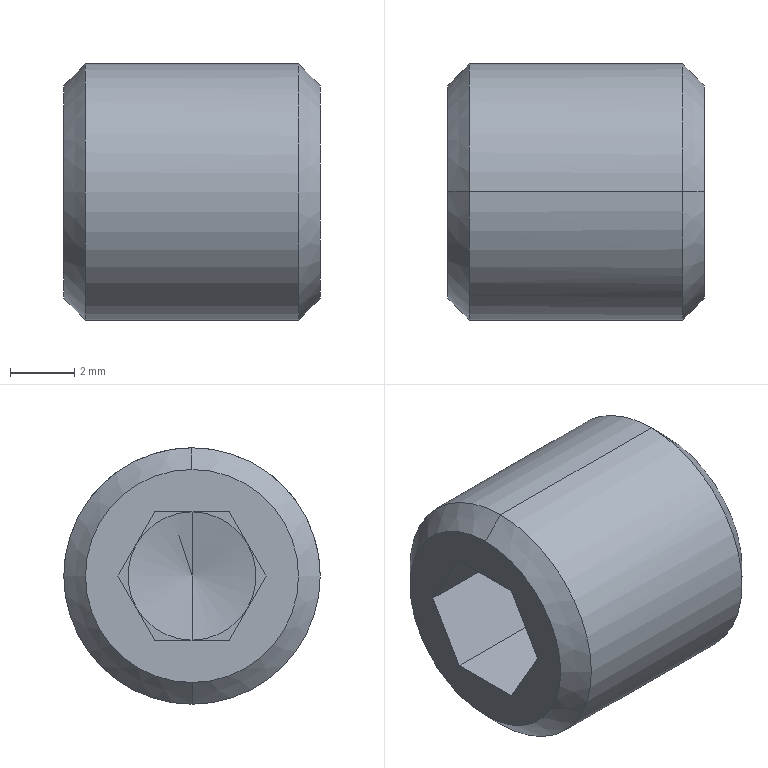Part | STEP file | _MSW8 | 1 solid | 22 faces | box 8 x 8 x 8 mm | volume 320.313 mm3 | plane 14 | cone 6 | cylinder 2 | commonest cylinder face diameters 8 x2
STEP:
#1=CARTESIAN_POINT('',(1.,0.,2.));
#2=VERTEX_POINT('',#1);
#3=CARTESIAN_POINT('',(1.,1.732,1.));
#4=VERTEX_POINT('',#3);
#5=CARTESIAN_POINT('',(1.,0.,0.));
#6=DIRECTION('',(-1.,0.,0.));
#7=AXIS2_PLACEMENT_3D('',#5,#6,$);
#8=CIRCLE('',#7,2.);
#9=EDGE_CURVE('',#2,#4,#8,.T.);
#10=ORIENTED_EDGE('',*,*,#9,.T.);
#11=CARTESIAN_POINT('',(1.,1.732,-1.));
#12=VERTEX_POINT('',#11);
#13=CARTESIAN_POINT('',(1.,0.,0.));
#14=DIRECTION('',(-1.,0.,0.));
#15=AXIS2_PLACEMENT_3D('',#13,#14,$);
#16=CIRCLE('',#15,2.);
#17=EDGE_CURVE('',#4,#12,#16,.T.);
#18=ORIENTED_EDGE('',*,*,#17,.T.);
#19=CARTESIAN_POINT('',(1.,0.,-2.));
#20=VERTEX_POINT('',#19);
#21=CARTESIAN_POINT('',(1.,0.,0.));
#22=DIRECTION('',(-1.,0.,0.));
#23=AXIS2_PLACEMENT_3D('',#21,#22,$);
#24=CIRCLE('',#23,2.);
#25=EDGE_CURVE('',#12,#20,#24,.T.);
#26=ORIENTED_EDGE('',*,*,#25,.T.);
#27=CARTESIAN_POINT('',(1.4,0.,0.));
#28=VERTEX_POINT('',#27);
#29=CARTESIAN_POINT('',(-98056.868,0.,-490291.338));
#30=DIRECTION('',(-0.1961,0.,-0.9806));
#31=VECTOR('',#30,1.);
#32=LINE('',#29,#31);
#33=EDGE_CURVE('',#28,#20,#32,.T.);
#34=ORIENTED_EDGE('',*,*,#33,.F.);
#35=CARTESIAN_POINT('',(-98056.868,0.,490291.338));
#36=DIRECTION('',(-0.1961,0.,0.9806));
#37=VECTOR('',#36,1.);
#38=LINE('',#35,#37);
#39=EDGE_CURVE('',#2,#28,#38,.F.);
#40=ORIENTED_EDGE('',*,*,#39,.F.);
#41=EDGE_LOOP('',(#10,#18,#26,#34,#40));
#42=FACE_OUTER_BOUND('',#41,.T.);
#43=CARTESIAN_POINT('',(1.,0.,0.));
#44=DIRECTION('',(-1.,0.,0.));
#45=DIRECTION('',(0.,0.,1.));
#46=AXIS2_PLACEMENT_3D('',#43,#44,#45);
#47=CONICAL_SURFACE('',#46,2.,1.373);
#48=ADVANCED_FACE('',(#42),#47,.F.);
#49=ORIENTED_EDGE('',*,*,#9,.F.);
#50=CARTESIAN_POINT('',(1.,1.155,2.));
#51=VERTEX_POINT('',#50);
#52=CARTESIAN_POINT('',(1.,0.5774,2.));
#53=DIRECTION('',(0.,-1.,0.));
#54=VECTOR('',#53,1.);
#55=LINE('',#52,#54);
#56=EDGE_CURVE('',#51,#2,#55,.T.);
#57=ORIENTED_EDGE('',*,*,#56,.F.);
#58=CARTESIAN_POINT('',(1.,1.443,1.5));
#59=DIRECTION('',(0.,-0.5,0.866));
#60=VECTOR('',#59,1.);
#61=LINE('',#58,#60);
#62=EDGE_CURVE('',#4,#51,#61,.T.);
#63=ORIENTED_EDGE('',*,*,#62,.F.);
#64=EDGE_LOOP('',(#49,#57,#63));
#65=FACE_OUTER_BOUND('',#64,.T.);
#66=CARTESIAN_POINT('',(1.,0.,0.));
#67=DIRECTION('',(1.,0.,0.));
#68=DIRECTION('',(0.,0.,-1.));
#69=AXIS2_PLACEMENT_3D('',#66,#67,#68);
#70=PLANE('',#69);
#71=ADVANCED_FACE('',(#65),#70,.F.);
#72=ORIENTED_EDGE('',*,*,#17,.F.);
#73=CARTESIAN_POINT('',(1.,2.309,0.));
#74=VERTEX_POINT('',#73);
#75=CARTESIAN_POINT('',(1.,2.021,0.5));
#76=DIRECTION('',(0.,-0.5,0.866));
#77=VECTOR('',#76,1.);
#78=LINE('',#75,#77);
#79=EDGE_CURVE('',#74,#4,#78,.T.);
#80=ORIENTED_EDGE('',*,*,#79,.F.);
#81=CARTESIAN_POINT('',(1.,2.021,-0.5));
#82=DIRECTION('',(0.,0.5,0.866));
#83=VECTOR('',#82,1.);
#84=LINE('',#81,#83);
#85=EDGE_CURVE('',#12,#74,#84,.T.);
#86=ORIENTED_EDGE('',*,*,#85,.F.);
#87=EDGE_LOOP('',(#72,#80,#86));
#88=FACE_OUTER_BOUND('',#87,.T.);
#89=CARTESIAN_POINT('',(1.,0.,0.));
#90=DIRECTION('',(1.,0.,0.));
#91=DIRECTION('',(0.,0.,-1.));
#92=AXIS2_PLACEMENT_3D('',#89,#90,#91);
#93=PLANE('',#92);
#94=ADVANCED_FACE('',(#88),#93,.F.);
#95=ORIENTED_EDGE('',*,*,#25,.F.);
#96=CARTESIAN_POINT('',(1.,1.155,-2.));
#97=VERTEX_POINT('',#96);
#98=CARTESIAN_POINT('',(1.,1.443,-1.5));
#99=DIRECTION('',(0.,0.5,0.866));
#100=VECTOR('',#99,1.);
#101=LINE('',#98,#100);
#102=EDGE_CURVE('',#97,#12,#101,.T.);
#103=ORIENTED_EDGE('',*,*,#102,.F.);
#104=CARTESIAN_POINT('',(1.,0.5774,-2.));
#105=DIRECTION('',(0.,1.,0.));
#106=VECTOR('',#105,1.);
#107=LINE('',#104,#106);
#108=EDGE_CURVE('',#20,#97,#107,.T.);
#109=ORIENTED_EDGE('',*,*,#108,.F.);
#110=EDGE_LOOP('',(#95,#103,#109));
#111=FACE_OUTER_BOUND('',#110,.T.);
#112=CARTESIAN_POINT('',(1.,0.,0.));
#113=DIRECTION('',(1.,0.,0.));
#114=DIRECTION('',(0.,0.,-1.));
#115=AXIS2_PLACEMENT_3D('',#112,#113,#114);
#116=PLANE('',#115);
#117=ADVANCED_FACE('',(#111),#116,.F.);
#118=CARTESIAN_POINT('',(1.,-1.732,-1.));
#119=VERTEX_POINT('',#118);
#120=CARTESIAN_POINT('',(1.,0.,0.));
#121=DIRECTION('',(-1.,0.,0.));
#122=AXIS2_PLACEMENT_3D('',#120,#121,$);
#123=CIRCLE('',#122,2.);
#124=EDGE_CURVE('',#20,#119,#123,.T.);
#125=ORIENTED_EDGE('',*,*,#124,.T.);
#126=CARTESIAN_POINT('',(1.,-1.732,1.));
#127=VERTEX_POINT('',#126);
#128=CARTESIAN_POINT('',(1.,0.,0.));
#129=DIRECTION('',(-1.,0.,0.));
#130=AXIS2_PLACEMENT_3D('',#128,#129,$);
#131=CIRCLE('',#130,2.);
#132=EDGE_CURVE('',#119,#127,#131,.T.);
#133=ORIENTED_EDGE('',*,*,#132,.T.);
#134=CARTESIAN_POINT('',(1.,0.,0.));
#135=DIRECTION('',(-1.,0.,0.));
#136=AXIS2_PLACEMENT_3D('',#134,#135,$);
#137=CIRCLE('',#136,2.);
#138=EDGE_CURVE('',#127,#2,#137,.T.);
#139=ORIENTED_EDGE('',*,*,#138,.T.);
#140=ORIENTED_EDGE('',*,*,#39,.T.);
#141=ORIENTED_EDGE('',*,*,#33,.T.);
#142=EDGE_LOOP('',(#125,#133,#139,#140,#141));
#143=FACE_OUTER_BOUND('',#142,.T.);
#144=CARTESIAN_POINT('',(1.,0.,0.));
#145=DIRECTION('',(-1.,0.,0.));
#146=DIRECTION('',(0.,0.,-1.));
#147=AXIS2_PLACEMENT_3D('',#144,#145,#146);
#148=CONICAL_SURFACE('',#147,2.,1.373);
#149=ADVANCED_FACE('',(#143),#148,.F.);
#150=CARTESIAN_POINT('',(-4.,1.155,2.));
#151=VERTEX_POINT('',#150);
#152=CARTESIAN_POINT('',(-4.,-1.155,2.));
#153=VERTEX_POINT('',#152);
#154=CARTESIAN_POINT('',(-4.,0.,2.));
#155=DIRECTION('',(0.,-1.,0.));
#156=VECTOR('',#155,1.);
#157=LINE('',#154,#156);
#158=EDGE_CURVE('',#151,#153,#157,.T.);
#159=ORIENTED_EDGE('',*,*,#158,.F.);
#160=CARTESIAN_POINT('',(-1.5,1.155,2.));
#161=DIRECTION('',(-1.,0.,0.));
#162=VECTOR('',#161,1.);
#163=LINE('',#160,#162);
#164=EDGE_CURVE('',#51,#151,#163,.T.);
#165=ORIENTED_EDGE('',*,*,#164,.F.);
#166=ORIENTED_EDGE('',*,*,#56,.T.);
#167=CARTESIAN_POINT('',(1.,-1.155,2.));
#168=VERTEX_POINT('',#167);
#169=CARTESIAN_POINT('',(1.,-0.5774,2.));
#170=DIRECTION('',(0.,-1.,0.));
#171=VECTOR('',#170,1.);
#172=LINE('',#169,#171);
#173=EDGE_CURVE('',#2,#168,#172,.T.);
#174=ORIENTED_EDGE('',*,*,#173,.T.);
#175=CARTESIAN_POINT('',(-1.5,-1.155,2.));
#176=DIRECTION('',(-1.,0.,0.));
#177=VECTOR('',#176,1.);
#178=LINE('',#175,#177);
#179=EDGE_CURVE('',#168,#153,#178,.T.);
#180=ORIENTED_EDGE('',*,*,#179,.T.);
#181=EDGE_LOOP('',(#159,#165,#166,#174,#180));
#182=FACE_OUTER_BOUND('',#181,.T.);
#183=CARTESIAN_POINT('',(1.,1.155,2.));
#184=DIRECTION('',(0.,0.,-1.));
#185=DIRECTION('',(-1.,0.,0.));
#186=AXIS2_PLACEMENT_3D('',#183,#184,#185);
#187=PLANE('',#186);
#188=ADVANCED_FACE('',(#182),#187,.T.);
#189=CARTESIAN_POINT('',(-4.,2.309,0.));
#190=VERTEX_POINT('',#189);
#191=CARTESIAN_POINT('',(-4.,1.732,1.));
#192=DIRECTION('',(0.,-0.5,0.866));
#193=VECTOR('',#192,1.);
#194=LINE('',#191,#193);
#195=EDGE_CURVE('',#190,#151,#194,.T.);
#196=ORIENTED_EDGE('',*,*,#195,.F.);
#197=CARTESIAN_POINT('',(-1.5,2.309,0.));
#198=DIRECTION('',(-1.,0.,0.));
#199=VECTOR('',#198,1.);
#200=LINE('',#197,#199);
#201=EDGE_CURVE('',#74,#190,#200,.T.);
#202=ORIENTED_EDGE('',*,*,#201,.F.);
#203=ORIENTED_EDGE('',*,*,#79,.T.);
#204=ORIENTED_EDGE('',*,*,#62,.T.);
#205=ORIENTED_EDGE('',*,*,#164,.T.);
#206=EDGE_LOOP('',(#196,#202,#203,#204,#205));
#207=FACE_OUTER_BOUND('',#206,.T.);
#208=CARTESIAN_POINT('',(1.,2.309,0.));
#209=DIRECTION('',(0.,-0.866,-0.5));
#210=DIRECTION('',(0.,0.5,-0.866));
#211=AXIS2_PLACEMENT_3D('',#208,#209,#210);
#212=PLANE('',#211);
#213=ADVANCED_FACE('',(#207),#212,.T.);
#214=CARTESIAN_POINT('',(-4.,1.155,-2.));
#215=VERTEX_POINT('',#214);
#216=CARTESIAN_POINT('',(-4.,1.732,-1.));
#217=DIRECTION('',(0.,0.5,0.866));
#218=VECTOR('',#217,1.);
#219=LINE('',#216,#218);
#220=EDGE_CURVE('',#215,#190,#219,.T.);
#221=ORIENTED_EDGE('',*,*,#220,.F.);
#222=CARTESIAN_POINT('',(-1.5,1.155,-2.));
#223=DIRECTION('',(-1.,0.,0.));
#224=VECTOR('',#223,1.);
#225=LINE('',#222,#224);
#226=EDGE_CURVE('',#97,#215,#225,.T.);
#227=ORIENTED_EDGE('',*,*,#226,.F.);
#228=ORIENTED_EDGE('',*,*,#102,.T.);
#229=ORIENTED_EDGE('',*,*,#85,.T.);
#230=ORIENTED_EDGE('',*,*,#201,.T.);
#231=EDGE_LOOP('',(#221,#227,#228,#229,#230));
#232=FACE_OUTER_BOUND('',#231,.T.);
#233=CARTESIAN_POINT('',(1.,1.155,-2.));
#234=DIRECTION('',(0.,-0.866,0.5));
#235=DIRECTION('',(0.,-0.5,-0.866));
#236=AXIS2_PLACEMENT_3D('',#233,#234,#235);
#237=PLANE('',#236);
#238=ADVANCED_FACE('',(#232),#237,.T.);
#239=CARTESIAN_POINT('',(-4.,-1.155,-2.));
#240=VERTEX_POINT('',#239);
#241=CARTESIAN_POINT('',(-4.,0.,-2.));
#242=DIRECTION('',(0.,1.,0.));
#243=VECTOR('',#242,1.);
#244=LINE('',#241,#243);
#245=EDGE_CURVE('',#240,#215,#244,.T.);
#246=ORIENTED_EDGE('',*,*,#245,.F.);
#247=CARTESIAN_POINT('',(1.,-1.155,-2.));
#248=VERTEX_POINT('',#247);
#249=CARTESIAN_POINT('',(-1.5,-1.155,-2.));
#250=DIRECTION('',(-1.,0.,0.));
#251=VECTOR('',#250,1.);
#252=LINE('',#249,#251);
#253=EDGE_CURVE('',#248,#240,#252,.T.);
#254=ORIENTED_EDGE('',*,*,#253,.F.);
#255=CARTESIAN_POINT('',(1.,-0.5774,-2.));
#256=DIRECTION('',(0.,1.,0.));
#257=VECTOR('',#256,1.);
#258=LINE('',#255,#257);
#259=EDGE_CURVE('',#248,#20,#258,.T.);
#260=ORIENTED_EDGE('',*,*,#259,.T.);
#261=ORIENTED_EDGE('',*,*,#108,.T.);
#262=ORIENTED_EDGE('',*,*,#226,.T.);
#263=EDGE_LOOP('',(#246,#254,#260,#261,#262));
#264=FACE_OUTER_BOUND('',#263,.T.);
#265=CARTESIAN_POINT('',(1.,-1.155,-2.));
#266=DIRECTION('',(0.,0.,1.));
#267=DIRECTION('',(1.,0.,0.));
#268=AXIS2_PLACEMENT_3D('',#265,#266,#267);
#269=PLANE('',#268);
#270=ADVANCED_FACE('',(#264),#269,.T.);
#271=ORIENTED_EDGE('',*,*,#124,.F.);
#272=ORIENTED_EDGE('',*,*,#259,.F.);
#273=CARTESIAN_POINT('',(1.,-1.443,-1.5));
#274=DIRECTION('',(0.,0.5,-0.866));
#275=VECTOR('',#274,1.);
#276=LINE('',#273,#275);
#277=EDGE_CURVE('',#119,#248,#276,.T.);
#278=ORIENTED_EDGE('',*,*,#277,.F.);
#279=EDGE_LOOP('',(#271,#272,#278));
#280=FACE_OUTER_BOUND('',#279,.T.);
#281=CARTESIAN_POINT('',(1.,0.,0.));
#282=DIRECTION('',(1.,0.,0.));
#283=DIRECTION('',(0.,0.,-1.));
#284=AXIS2_PLACEMENT_3D('',#281,#282,#283);
#285=PLANE('',#284);
#286=ADVANCED_FACE('',(#280),#285,.F.);
#287=ORIENTED_EDGE('',*,*,#132,.F.);
#288=CARTESIAN_POINT('',(1.,-2.309,0.));
#289=VERTEX_POINT('',#288);
#290=CARTESIAN_POINT('',(1.,-2.021,-0.5));
#291=DIRECTION('',(0.,0.5,-0.866));
#292=VECTOR('',#291,1.);
#293=LINE('',#290,#292);
#294=EDGE_CURVE('',#289,#119,#293,.T.);
#295=ORIENTED_EDGE('',*,*,#294,.F.);
#296=CARTESIAN_POINT('',(1.,-2.021,0.5));
#297=DIRECTION('',(0.,-0.5,-0.866));
#298=VECTOR('',#297,1.);
#299=LINE('',#296,#298);
#300=EDGE_CURVE('',#127,#289,#299,.T.);
#301=ORIENTED_EDGE('',*,*,#300,.F.);
#302=EDGE_LOOP('',(#287,#295,#301));
#303=FACE_OUTER_BOUND('',#302,.T.);
#304=CARTESIAN_POINT('',(1.,0.,0.));
#305=DIRECTION('',(1.,0.,0.));
#306=DIRECTION('',(0.,0.,-1.));
#307=AXIS2_PLACEMENT_3D('',#304,#305,#306);
#308=PLANE('',#307);
#309=ADVANCED_FACE('',(#303),#308,.F.);
#310=ORIENTED_EDGE('',*,*,#138,.F.);
#311=CARTESIAN_POINT('',(1.,-1.443,1.5));
#312=DIRECTION('',(0.,-0.5,-0.866));
#313=VECTOR('',#312,1.);
#314=LINE('',#311,#313);
#315=EDGE_CURVE('',#168,#127,#314,.T.);
#316=ORIENTED_EDGE('',*,*,#315,.F.);
#317=ORIENTED_EDGE('',*,*,#173,.F.);
#318=EDGE_LOOP('',(#310,#316,#317));
#319=FACE_OUTER_BOUND('',#318,.T.);
#320=CARTESIAN_POINT('',(1.,0.,0.));
#321=DIRECTION('',(1.,0.,0.));
#322=DIRECTION('',(0.,0.,-1.));
#323=AXIS2_PLACEMENT_3D('',#320,#321,#322);
#324=PLANE('',#323);
#325=ADVANCED_FACE('',(#319),#324,.F.);
#326=CARTESIAN_POINT('',(-4.,0.,-3.324));
#327=VERTEX_POINT('',#326);
#328=CARTESIAN_POINT('',(-4.,3.324,0.));
#329=VERTEX_POINT('',#328);
#330=CARTESIAN_POINT('',(-4.,0.,0.));
#331=DIRECTION('',(1.,0.,0.));
#332=AXIS2_PLACEMENT_3D('',#330,#331,$);
#333=CIRCLE('',#332,3.323);
#334=EDGE_CURVE('',#327,#329,#333,.T.);
#335=ORIENTED_EDGE('',*,*,#334,.F.);
#336=CARTESIAN_POINT('',(-4.,-3.324,0.));
#337=VERTEX_POINT('',#336);
#338=CARTESIAN_POINT('',(-4.,0.,0.));
#339=DIRECTION('',(1.,0.,0.));
#340=AXIS2_PLACEMENT_3D('',#338,#339,$);
#341=CIRCLE('',#340,3.323);
#342=EDGE_CURVE('',#337,#327,#341,.T.);
#343=ORIENTED_EDGE('',*,*,#342,.F.);
#344=CARTESIAN_POINT('',(-4.,0.,3.324));
#345=VERTEX_POINT('',#344);
#346=CARTESIAN_POINT('',(-4.,0.,0.));
#347=DIRECTION('',(1.,0.,0.));
#348=AXIS2_PLACEMENT_3D('',#346,#347,$);
#349=CIRCLE('',#348,3.323);
#350=EDGE_CURVE('',#345,#337,#349,.T.);
#351=ORIENTED_EDGE('',*,*,#350,.F.);
#352=CARTESIAN_POINT('',(-4.,0.,0.));
#353=DIRECTION('',(1.,0.,0.));
#354=AXIS2_PLACEMENT_3D('',#352,#353,$);
#355=CIRCLE('',#354,3.323);
#356=EDGE_CURVE('',#329,#345,#355,.T.);
#357=ORIENTED_EDGE('',*,*,#356,.F.);
#358=EDGE_LOOP('',(#335,#343,#351,#357));
#359=FACE_OUTER_BOUND('',#358,.T.);
#360=ORIENTED_EDGE('',*,*,#158,.T.);
#361=CARTESIAN_POINT('',(-4.,-2.309,0.));
#362=VERTEX_POINT('',#361);
#363=CARTESIAN_POINT('',(-4.,-1.732,1.));
#364=DIRECTION('',(0.,-0.5,-0.866));
#365=VECTOR('',#364,1.);
#366=LINE('',#363,#365);
#367=EDGE_CURVE('',#153,#362,#366,.T.);
#368=ORIENTED_EDGE('',*,*,#367,.T.);
#369=CARTESIAN_POINT('',(-4.,-1.732,-1.));
#370=DIRECTION('',(0.,0.5,-0.866));
#371=VECTOR('',#370,1.);
#372=LINE('',#369,#371);
#373=EDGE_CURVE('',#362,#240,#372,.T.);
#374=ORIENTED_EDGE('',*,*,#373,.T.);
#375=ORIENTED_EDGE('',*,*,#245,.T.);
#376=ORIENTED_EDGE('',*,*,#220,.T.);
#377=ORIENTED_EDGE('',*,*,#195,.T.);
#378=EDGE_LOOP('',(#360,#368,#374,#375,#376,#377));
#379=FACE_BOUND('',#378,.T.);
#380=CARTESIAN_POINT('',(-4.,0.,0.));
#381=DIRECTION('',(1.,0.,0.));
#382=DIRECTION('',(0.,0.,-1.));
#383=AXIS2_PLACEMENT_3D('',#380,#381,#382);
#384=PLANE('',#383);
#385=ADVANCED_FACE('',(#359,#379),#384,.F.);
#386=ORIENTED_EDGE('',*,*,#367,.F.);
#387=ORIENTED_EDGE('',*,*,#179,.F.);
#388=ORIENTED_EDGE('',*,*,#315,.T.);
#389=ORIENTED_EDGE('',*,*,#300,.T.);
#390=CARTESIAN_POINT('',(-1.5,-2.309,0.));
#391=DIRECTION('',(-1.,0.,0.));
#392=VECTOR('',#391,1.);
#393=LINE('',#390,#392);
#394=EDGE_CURVE('',#289,#362,#393,.T.);
#395=ORIENTED_EDGE('',*,*,#394,.T.);
#396=EDGE_LOOP('',(#386,#387,#388,#389,#395));
#397=FACE_OUTER_BOUND('',#396,.T.);
#398=CARTESIAN_POINT('',(1.,-1.155,2.));
#399=DIRECTION('',(0.,0.866,-0.5));
#400=DIRECTION('',(0.,0.5,0.866));
#401=AXIS2_PLACEMENT_3D('',#398,#399,#400);
#402=PLANE('',#401);
#403=ADVANCED_FACE('',(#397),#402,.T.);
#404=ORIENTED_EDGE('',*,*,#373,.F.);
#405=ORIENTED_EDGE('',*,*,#394,.F.);
#406=ORIENTED_EDGE('',*,*,#294,.T.);
#407=ORIENTED_EDGE('',*,*,#277,.T.);
#408=ORIENTED_EDGE('',*,*,#253,.T.);
#409=EDGE_LOOP('',(#404,#405,#406,#407,#408));
#410=FACE_OUTER_BOUND('',#409,.T.);
#411=CARTESIAN_POINT('',(1.,-2.309,0.));
#412=DIRECTION('',(0.,0.866,0.5));
#413=DIRECTION('',(0.,-0.5,0.866));
#414=AXIS2_PLACEMENT_3D('',#411,#412,#413);
#415=PLANE('',#414);
#416=ADVANCED_FACE('',(#410),#415,.T.);
#417=CARTESIAN_POINT('',(-3.323,0.,-4.));
#418=VERTEX_POINT('',#417);
#419=CARTESIAN_POINT('',(353547.729,0.,-353555.052));
#420=DIRECTION('',(0.7071,0.,-0.7071));
#421=VECTOR('',#420,1.);
#422=LINE('',#419,#421);
#423=EDGE_CURVE('',#418,#327,#422,.F.);
#424=ORIENTED_EDGE('',*,*,#423,.T.);
#425=ORIENTED_EDGE('',*,*,#334,.T.);
#426=ORIENTED_EDGE('',*,*,#356,.T.);
#427=CARTESIAN_POINT('',(-3.324,0.,4.));
#428=VERTEX_POINT('',#427);
#429=CARTESIAN_POINT('',(353547.729,0.,353555.052));
#430=DIRECTION('',(0.7071,0.,0.7071));
#431=VECTOR('',#430,1.);
#432=LINE('',#429,#431);
#433=EDGE_CURVE('',#345,#428,#432,.T.);
#434=ORIENTED_EDGE('',*,*,#433,.T.);
#435=CARTESIAN_POINT('',(-3.323,4.,0.));
#436=VERTEX_POINT('',#435);
#437=CARTESIAN_POINT('',(-3.324,0.,0.));
#438=DIRECTION('',(1.,0.,0.));
#439=AXIS2_PLACEMENT_3D('',#437,#438,$);
#440=CIRCLE('',#439,4.);
#441=EDGE_CURVE('',#436,#428,#440,.T.);
#442=ORIENTED_EDGE('',*,*,#441,.F.);
#443=CARTESIAN_POINT('',(-3.324,0.,0.));
#444=DIRECTION('',(1.,0.,0.));
#445=AXIS2_PLACEMENT_3D('',#443,#444,$);
#446=CIRCLE('',#445,4.);
#447=EDGE_CURVE('',#418,#436,#446,.T.);
#448=ORIENTED_EDGE('',*,*,#447,.F.);
#449=EDGE_LOOP('',(#424,#425,#426,#434,#442,#448));
#450=FACE_OUTER_BOUND('',#449,.T.);
#451=CARTESIAN_POINT('',(-4.,0.,0.));
#452=DIRECTION('',(1.,0.,0.));
#453=DIRECTION('',(0.,0.,-1.));
#454=AXIS2_PLACEMENT_3D('',#451,#452,#453);
#455=CONICAL_SURFACE('',#454,3.324,0.7854);
#456=ADVANCED_FACE('',(#450),#455,.T.);
#457=ORIENTED_EDGE('',*,*,#433,.F.);
#458=ORIENTED_EDGE('',*,*,#350,.T.);
#459=ORIENTED_EDGE('',*,*,#342,.T.);
#460=ORIENTED_EDGE('',*,*,#423,.F.);
#461=CARTESIAN_POINT('',(-3.324,-4.,0.));
#462=VERTEX_POINT('',#461);
#463=CARTESIAN_POINT('',(-3.324,0.,0.));
#464=DIRECTION('',(1.,0.,0.));
#465=AXIS2_PLACEMENT_3D('',#463,#464,$);
#466=CIRCLE('',#465,4.);
#467=EDGE_CURVE('',#462,#418,#466,.T.);
#468=ORIENTED_EDGE('',*,*,#467,.F.);
#469=CARTESIAN_POINT('',(-3.324,0.,0.));
#470=DIRECTION('',(1.,0.,0.));
#471=AXIS2_PLACEMENT_3D('',#469,#470,$);
#472=CIRCLE('',#471,4.);
#473=EDGE_CURVE('',#428,#462,#472,.T.);
#474=ORIENTED_EDGE('',*,*,#473,.F.);
#475=EDGE_LOOP('',(#457,#458,#459,#460,#468,#474));
#476=FACE_OUTER_BOUND('',#475,.T.);
#477=CARTESIAN_POINT('',(-4.,0.,0.));
#478=DIRECTION('',(1.,0.,0.));
#479=DIRECTION('',(0.,0.,1.));
#480=AXIS2_PLACEMENT_3D('',#477,#478,#479);
#481=CONICAL_SURFACE('',#480,3.324,0.7854);
#482=ADVANCED_FACE('',(#476),#481,.T.);
#483=CARTESIAN_POINT('',(3.324,0.,-4.));
#484=VERTEX_POINT('',#483);
#485=CARTESIAN_POINT('',(4.,0.,-4.));
#486=DIRECTION('',(-1.,0.,0.));
#487=VECTOR('',#486,1.);
#488=LINE('',#485,#487);
#489=EDGE_CURVE('',#418,#484,#488,.F.);
#490=ORIENTED_EDGE('',*,*,#489,.F.);
#491=ORIENTED_EDGE('',*,*,#447,.T.);
#492=ORIENTED_EDGE('',*,*,#441,.T.);
#493=CARTESIAN_POINT('',(3.324,0.,4.));
#494=VERTEX_POINT('',#493);
#495=CARTESIAN_POINT('',(4.,0.,4.));
#496=DIRECTION('',(-1.,0.,0.));
#497=VECTOR('',#496,1.);
#498=LINE('',#495,#497);
#499=EDGE_CURVE('',#494,#428,#498,.T.);
#500=ORIENTED_EDGE('',*,*,#499,.F.);
#501=CARTESIAN_POINT('',(3.324,4.,0.));
#502=VERTEX_POINT('',#501);
#503=CARTESIAN_POINT('',(3.323,4.,0.));
#504=CARTESIAN_POINT('',(3.323,4.,1.257));
#505=CARTESIAN_POINT('',(3.323,3.508,2.514));
#506=CARTESIAN_POINT('',(3.323,2.514,3.508));
#507=CARTESIAN_POINT('',(3.323,1.257,4.));
#508=CARTESIAN_POINT('',(3.324,0.,4.));
#509=B_SPLINE_CURVE_WITH_KNOTS('',5,(#503,#504,#505,#506,#507,#508),.UNSPECIFIED.,.F.,.U.,(6,6),(-3.142,3.142),.UNSPECIFIED.);
#510=EDGE_CURVE('',#502,#494,#509,.T.);
#511=ORIENTED_EDGE('',*,*,#510,.F.);
#512=CARTESIAN_POINT('',(3.323,0.,0.));
#513=DIRECTION('',(-1.,0.,0.));
#514=AXIS2_PLACEMENT_3D('',#512,#513,$);
#515=CIRCLE('',#514,4.);
#516=EDGE_CURVE('',#484,#502,#515,.F.);
#517=ORIENTED_EDGE('',*,*,#516,.F.);
#518=EDGE_LOOP('',(#490,#491,#492,#500,#511,#517));
#519=FACE_OUTER_BOUND('',#518,.T.);
#520=CARTESIAN_POINT('',(4.,0.,0.));
#521=DIRECTION('',(-1.,0.,0.));
#522=DIRECTION('',(0.,0.,1.));
#523=AXIS2_PLACEMENT_3D('',#520,#521,#522);
#524=CYLINDRICAL_SURFACE('',#523,4.);
#525=ADVANCED_FACE('',(#519),#524,.T.);
#526=ORIENTED_EDGE('',*,*,#499,.T.);
#527=ORIENTED_EDGE('',*,*,#473,.T.);
#528=ORIENTED_EDGE('',*,*,#467,.T.);
#529=ORIENTED_EDGE('',*,*,#489,.T.);
#530=CARTESIAN_POINT('',(3.324,-4.,0.));
#531=VERTEX_POINT('',#530);
#532=CARTESIAN_POINT('',(3.323,0.,0.));
#533=DIRECTION('',(-1.,0.,0.));
#534=AXIS2_PLACEMENT_3D('',#532,#533,$);
#535=CIRCLE('',#534,4.);
#536=EDGE_CURVE('',#531,#484,#535,.F.);
#537=ORIENTED_EDGE('',*,*,#536,.F.);
#538=CARTESIAN_POINT('',(3.324,0.,4.));
#539=CARTESIAN_POINT('',(3.323,-1.257,4.));
#540=CARTESIAN_POINT('',(3.323,-2.514,3.508));
#541=CARTESIAN_POINT('',(3.323,-3.508,2.514));
#542=CARTESIAN_POINT('',(3.323,-4.,1.257));
#543=CARTESIAN_POINT('',(3.323,-4.,0.));
#544=B_SPLINE_CURVE_WITH_KNOTS('',5,(#538,#539,#540,#541,#542,#543),.UNSPECIFIED.,.F.,.U.,(6,6),(-3.142,3.142),.UNSPECIFIED.);
#545=EDGE_CURVE('',#494,#531,#544,.T.);
#546=ORIENTED_EDGE('',*,*,#545,.F.);
#547=EDGE_LOOP('',(#526,#527,#528,#529,#537,#546));
#548=FACE_OUTER_BOUND('',#547,.T.);
#549=CARTESIAN_POINT('',(4.,0.,0.));
#550=DIRECTION('',(-1.,0.,0.));
#551=DIRECTION('',(0.,0.,-1.));
#552=AXIS2_PLACEMENT_3D('',#549,#550,#551);
#553=CYLINDRICAL_SURFACE('',#552,4.);
#554=ADVANCED_FACE('',(#548),#553,.T.);
#555=CARTESIAN_POINT('',(4.,0.,3.324));
#556=VERTEX_POINT('',#555);
#557=CARTESIAN_POINT('',(-353548.067,0.,353555.391));
#558=DIRECTION('',(-0.7071,0.,0.7071));
#559=VECTOR('',#558,1.);
#560=LINE('',#557,#559);
#561=EDGE_CURVE('',#494,#556,#560,.F.);
#562=ORIENTED_EDGE('',*,*,#561,.T.);
#563=CARTESIAN_POINT('',(4.,3.324,0.));
#564=VERTEX_POINT('',#563);
#565=CARTESIAN_POINT('',(4.,0.,0.));
#566=DIRECTION('',(-1.,0.,0.));
#567=AXIS2_PLACEMENT_3D('',#565,#566,$);
#568=CIRCLE('',#567,3.324);
#569=EDGE_CURVE('',#564,#556,#568,.F.);
#570=ORIENTED_EDGE('',*,*,#569,.F.);
#571=CARTESIAN_POINT('',(4.,0.,-3.324));
#572=VERTEX_POINT('',#571);
#573=CARTESIAN_POINT('',(4.,0.,0.));
#574=DIRECTION('',(-1.,0.,0.));
#575=AXIS2_PLACEMENT_3D('',#573,#574,$);
#576=CIRCLE('',#575,3.324);
#577=EDGE_CURVE('',#572,#564,#576,.F.);
#578=ORIENTED_EDGE('',*,*,#577,.F.);
#579=CARTESIAN_POINT('',(-353548.067,0.,-353555.391));
#580=DIRECTION('',(-0.7071,0.,-0.7071));
#581=VECTOR('',#580,1.);
#582=LINE('',#579,#581);
#583=EDGE_CURVE('',#572,#484,#582,.T.);
#584=ORIENTED_EDGE('',*,*,#583,.T.);
#585=ORIENTED_EDGE('',*,*,#516,.T.);
#586=ORIENTED_EDGE('',*,*,#510,.T.);
#587=EDGE_LOOP('',(#562,#570,#578,#584,#585,#586));
#588=FACE_OUTER_BOUND('',#587,.T.);
#589=CARTESIAN_POINT('',(3.324,0.,0.));
#590=DIRECTION('',(-1.,0.,0.));
#591=DIRECTION('',(0.,0.,1.));
#592=AXIS2_PLACEMENT_3D('',#589,#590,#591);
#593=CONICAL_SURFACE('',#592,4.,0.7854);
#594=ADVANCED_FACE('',(#588),#593,.T.);
#595=ORIENTED_EDGE('',*,*,#583,.F.);
#596=CARTESIAN_POINT('',(4.,-3.324,0.));
#597=VERTEX_POINT('',#596);
#598=CARTESIAN_POINT('',(4.,0.,0.));
#599=DIRECTION('',(-1.,0.,0.));
#600=AXIS2_PLACEMENT_3D('',#598,#599,$);
#601=CIRCLE('',#600,3.324);
#602=EDGE_CURVE('',#597,#572,#601,.F.);
#603=ORIENTED_EDGE('',*,*,#602,.F.);
#604=CARTESIAN_POINT('',(4.,0.,0.));
#605=DIRECTION('',(-1.,0.,0.));
#606=AXIS2_PLACEMENT_3D('',#604,#605,$);
#607=CIRCLE('',#606,3.324);
#608=EDGE_CURVE('',#556,#597,#607,.F.);
#609=ORIENTED_EDGE('',*,*,#608,.F.);
#610=ORIENTED_EDGE('',*,*,#561,.F.);
#611=ORIENTED_EDGE('',*,*,#545,.T.);
#612=ORIENTED_EDGE('',*,*,#536,.T.);
#613=EDGE_LOOP('',(#595,#603,#609,#610,#611,#612));
#614=FACE_OUTER_BOUND('',#613,.T.);
#615=CARTESIAN_POINT('',(3.324,0.,0.));
#616=DIRECTION('',(-1.,0.,0.));
#617=DIRECTION('',(0.,0.,-1.));
#618=AXIS2_PLACEMENT_3D('',#615,#616,#617);
#619=CONICAL_SURFACE('',#618,4.,0.7854);
#620=ADVANCED_FACE('',(#614),#619,.T.);
#621=ORIENTED_EDGE('',*,*,#569,.T.);
#622=ORIENTED_EDGE('',*,*,#608,.T.);
#623=ORIENTED_EDGE('',*,*,#602,.T.);
#624=ORIENTED_EDGE('',*,*,#577,.T.);
#625=EDGE_LOOP('',(#621,#622,#623,#624));
#626=FACE_OUTER_BOUND('',#625,.T.);
#627=CARTESIAN_POINT('',(4.,3.324,0.));
#628=DIRECTION('',(-1.,0.,0.));
#629=DIRECTION('',(0.,0.,1.));
#630=AXIS2_PLACEMENT_3D('',#627,#628,#629);
#631=PLANE('',#630);
#632=ADVANCED_FACE('',(#626),#631,.F.);
#633=CLOSED_SHELL('',(#48,#71,#94,#117,#149,#188,#213,#238,#270,#286,#309,#325,#385,#403,#416,#456,#482,#525,#554,#594,#620,#632));
#634=MANIFOLD_SOLID_BREP('',#633);
#635=(LENGTH_UNIT()NAMED_UNIT(*)SI_UNIT(.MILLI.,.METRE.));
#636=UNCERTAINTY_MEASURE_WITH_UNIT(LENGTH_MEASURE(0.005),#635,'','');
#637=(NAMED_UNIT(*)PLANE_ANGLE_UNIT()SI_UNIT($,.RADIAN.));
#638=(NAMED_UNIT(*)SI_UNIT($,.STERADIAN.)SOLID_ANGLE_UNIT());
#639=(GEOMETRIC_REPRESENTATION_CONTEXT(3)GLOBAL_UNCERTAINTY_ASSIGNED_CONTEXT((#636))GLOBAL_UNIT_ASSIGNED_CONTEXT((#635,#637,#638))REPRESENTATION_CONTEXT('',''));
#640=ADVANCED_BREP_SHAPE_REPRESENTATION('',(#634),#639);